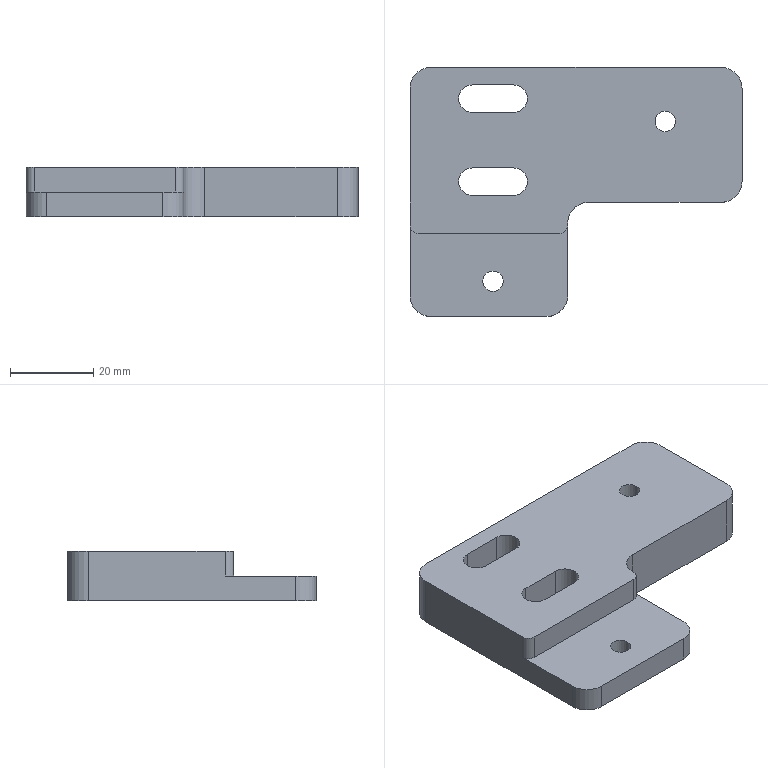NC program | NX | posted with a generic post | part box 80 x 60 x 12 mm
Lines 2006 to 2096 of 5338:
(ZLEVEL_PROFILE_COPY_1 , TOOL : D10JING)
N3998 T14 M6
N4000 G54
N4002 G17 G0 G90 X40.672 Y33.213 S9500 M3
N4004 G43 Z30. H14
N4006 Z1.5
N4008 G94 G1 X41.34 Y32.772 Z1.458 F1000.
N4010 X42.772 Y31.34 Z1.352
N4012 X43.887 Y29.649 Z1.246
N4014 X44.64 Y27.769 Z1.14
N4016 X45. Y25.775 Z1.033
N4018 Y1.725 Z-0.227
N4020 X44.64 Y-0.269 Z-0.333
N4022 X43.887 Y-2.149 Z-0.439
N4024 X42.772 Y-3.84 Z-0.545
N4026 X41.34 Y-5.272 Z-0.652
N4028 X39.649 Y-6.387 Z-0.758
N4030 X37.769 Y-7.14 Z-0.864
N4032 X35.775 Y-7.5 Z-0.97
N4034 X3. Z-2.688
N4036 Y-25.775 Z-3.646
N4038 X2.64 Y-27.769 Z-3.752
N4040 X1.887 Y-29.649 Z-3.858
N4042 X0.772 Y-31.34 Z-3.964
N4044 X-0.66 Y-32.772 Z-4.07
N4046 X-2.351 Y-33.887 Z-4.176
N4048 X-4.231 Y-34.64 Z-4.282
N4050 X-6.225 Y-35. Z-4.389
N4052 X-35.775 Z-5.937
N4054 X-37.769 Y-34.64 Z-6.043
N4056 X-39.649 Y-33.887 Z-6.15
N4058 X-41.34 Y-32.772 Z-6.256
N4060 X-42.772 Y-31.34 Z-6.362
N4062 X-43.887 Y-29.649 Z-6.468
N4064 X-44.64 Y-27.769 Z-6.574
N4066 X-45. Y-25.775 Z-6.68
N4068 Y25.775 Z-9.382
N4070 X-44.64 Y27.769 Z-9.488
N4072 X-43.887 Y29.649 Z-9.594
N4074 X-42.772 Y31.34 Z-9.7
N4076 X-41.34 Y32.772 Z-9.807
N4078 X-39.649 Y33.887 Z-9.913
N4080 X-37.769 Y34.64 Z-10.019
N4082 X-35.775 Y35. Z-10.125
N4084 X0. Z-12.
N4086 X35. F1200.
N4088 G2 X45. Y25. R10.
N4090 G1 Y2.5
N4092 G2 X35. Y-7.5 R10.
N4094 G1 X3.
N4096 Y-25.
N4098 G2 X-7. Y-35. R10.
N4100 G1 X-35.
N4102 G2 X-45. Y-25. R10.
N4104 G1 Y25.
N4106 G2 X-35. Y35. R10.
N4108 G1 X0.
N4110 Z-10.5
N4112 G0 Z30.
(FLOOR_WALL_2 , TOOL : D10JING)
N4114 X-48. Y-15.503
N4116 Z-3.
N4118 G1 Z-6. F1500.
N4120 X-45.
N4122 X3.
N4124 Y-19.002
N4126 X-45.
N4128 Y-22.501
N4130 X3.
N4132 Y-25.
N4134 G2 X2.95 Y-26. R10.
N4136 G1 X-44.95
N4138 X-47.961
N4140 Z-3.
N4142 G0 Z30.
N4144 X6. Y-10.5
N4146 Z-3.
N4148 G1 Z-6.
N4150 X2.97 Y-8.647
N4152 G2 X-4. Y-15. R7.
N4154 G1 X-38.
N4156 G2 X-44.97 Y-8.647 R7.
N4158 G1 X-45.247 Y-5.66
N4160 X-48.
N4162 Z-3.
N4164 G0 Z30.
N4166 M5